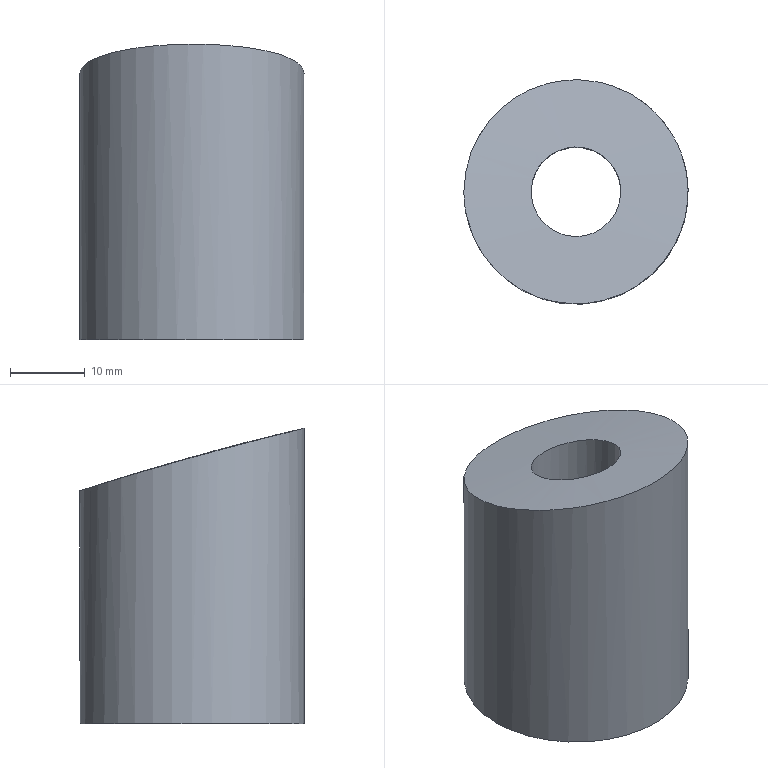Part | NX | features solid 2 | 1 solid | 4 faces | box 30.001 x 30 x 39.543 mm | volume 21121 mm3 | cylinder 2 | spline 1 | plane 1 | commonest cylinder face diameters 12 x1 30 x1
STEP:
#1=CARTESIAN_POINT('',(-749.977,149.178,105.858));
#2=VERTEX_POINT('',#1);
#3=CARTESIAN_POINT('',(-747.09,139.627,108.386));
#4=CARTESIAN_POINT('',(-751.538,149.125,105.94));
#5=CARTESIAN_POINT('',(-748.183,158.887,103.085));
#6=CARTESIAN_POINT('',(-741.846,163.791,101.556));
#7=CARTESIAN_POINT('',(-735.95,165.378,101.05));
#8=CARTESIAN_POINT('',(-729.883,164.528,101.326));
#9=CARTESIAN_POINT('',(-722.94,160.384,102.647));
#10=CARTESIAN_POINT('',(-718.485,151.039,105.473));
#11=CARTESIAN_POINT('',(-721.752,141.177,108.077));
#12=CARTESIAN_POINT('',(-728.129,136.217,109.277));
#13=CARTESIAN_POINT('',(-734.033,134.622,109.636));
#14=CARTESIAN_POINT('',(-740.114,135.47,109.413));
#15=CARTESIAN_POINT('',(-747.09,139.627,108.386));
#16=CARTESIAN_POINT('',(-751.538,149.125,105.94));
#17=CARTESIAN_POINT('',(-748.183,158.887,103.085));
#18=B_SPLINE_CURVE_WITH_KNOTS('',3,(#3,#4,#5,#6,#7,#8,#9,#10,#11,#12,#13,#14,#15,#16,#17),.UNSPECIFIED.,.T.,.F.,(1,1,1,1,1,1,1,1,1,1,1,1,1,1,1,1,1,1,1),(-0.02388,-0.01791,-0.01194,0.,0.01194,0.01791,0.02388,0.02986,0.03583,0.04777,0.05971,0.06568,0.07165,0.07762,0.0836,0.09554,0.1075,0.1135,0.1194),.UNSPECIFIED.);
#19=EDGE_CURVE('',#2,#2,#18,.T.);
#20=ORIENTED_EDGE('',*,*,#19,.T.);
#21=EDGE_LOOP('',(#20));
#22=FACE_BOUND('',#21,.T.);
#23=CARTESIAN_POINT('',(-750.,150.,70.));
#24=VERTEX_POINT('',#23);
#25=CARTESIAN_POINT('',(-735.,150.,70.));
#26=DIRECTION('',(0.,0.,-1.));
#27=DIRECTION('',(-1.,0.,0.));
#28=AXIS2_PLACEMENT_3D('',#25,#26,#27);
#29=CIRCLE('',#28,15.);
#30=EDGE_CURVE('',#24,#24,#29,.T.);
#31=ORIENTED_EDGE('',*,*,#30,.F.);
#32=EDGE_LOOP('',(#31));
#33=FACE_BOUND('',#32,.T.);
#34=CARTESIAN_POINT('',(-735.,150.,120.));
#35=DIRECTION('',(0.,0.,-1.));
#36=DIRECTION('',(-1.,0.,0.));
#37=AXIS2_PLACEMENT_3D('',#34,#35,#36);
#38=CYLINDRICAL_SURFACE('',#37,15.);
#39=ADVANCED_FACE('',(#22,#33),#38,.T.);
#40=CARTESIAN_POINT('',(-729.,150.,105.676));
#41=VERTEX_POINT('',#40);
#42=CARTESIAN_POINT('',(-730.23,154.633,104.356));
#43=CARTESIAN_POINT('',(-728.384,150.001,105.688));
#44=CARTESIAN_POINT('',(-730.235,145.362,106.945));
#45=CARTESIAN_POINT('',(-735.002,143.317,107.465));
#46=CARTESIAN_POINT('',(-739.777,145.37,106.918));
#47=CARTESIAN_POINT('',(-741.615,150.02,105.656));
#48=CARTESIAN_POINT('',(-739.764,154.633,104.342));
#49=CARTESIAN_POINT('',(-735.004,156.684,103.739));
#50=CARTESIAN_POINT('',(-730.23,154.633,104.356));
#51=CARTESIAN_POINT('',(-728.384,150.001,105.688));
#52=CARTESIAN_POINT('',(-730.235,145.362,106.945));
#53=B_SPLINE_CURVE_WITH_KNOTS('',3,(#42,#43,#44,#45,#46,#47,#48,#49,#50,#51,#52),.UNSPECIFIED.,.T.,.F.,(1,1,1,1,1,1,1,1,1,1,1,1,1,1,1),(-0.01433,-0.009554,-0.004777,0.,0.004777,0.009554,0.01433,0.01911,0.02389,0.02866,0.03344,0.03822,0.04299,0.04777,0.05255),.UNSPECIFIED.);
#54=EDGE_CURVE('',#41,#41,#53,.T.);
#55=ORIENTED_EDGE('',*,*,#54,.T.);
#56=EDGE_LOOP('',(#55));
#57=FACE_BOUND('',#56,.T.);
#58=ORIENTED_EDGE('',*,*,#19,.F.);
#59=EDGE_LOOP('',(#58));
#60=FACE_BOUND('',#59,.T.);
#61=CARTESIAN_POINT('',(-751.476,165.919,100.866));
#62=CARTESIAN_POINT('',(-750.684,155.902,104.088));
#63=CARTESIAN_POINT('',(-749.909,145.712,106.935));
#64=CARTESIAN_POINT('',(-749.151,135.347,109.408));
#65=CARTESIAN_POINT('',(-741.263,165.51,101.003));
#66=CARTESIAN_POINT('',(-740.466,155.482,104.226));
#67=CARTESIAN_POINT('',(-739.686,145.281,107.076));
#68=CARTESIAN_POINT('',(-738.924,134.905,109.55));
#69=CARTESIAN_POINT('',(-731.05,165.1,101.14));
#70=CARTESIAN_POINT('',(-730.248,155.062,104.365));
#71=CARTESIAN_POINT('',(-729.464,144.85,107.216));
#72=CARTESIAN_POINT('',(-728.698,134.463,109.692));
#73=CARTESIAN_POINT('',(-720.837,164.691,101.277));
#74=CARTESIAN_POINT('',(-720.031,154.642,104.504));
#75=CARTESIAN_POINT('',(-719.242,144.419,107.356));
#76=CARTESIAN_POINT('',(-718.471,134.021,109.834));
#77=B_SPLINE_SURFACE_WITH_KNOTS('',3,3,((#61,#62,#63,#64),(#65,#66,#67,#68),(#69,#70,#71,#72),(#73,#74,#75,#76)),.UNSPECIFIED.,.F.,.F.,.F.,(4,4),(4,4),(0.2165,0.6205),(0.479,0.7331),.UNSPECIFIED.);
#78=ADVANCED_FACE('',(#57,#60),#77,.F.);
#79=CARTESIAN_POINT('',(-729.,150.,70.));
#80=VERTEX_POINT('',#79);
#81=CARTESIAN_POINT('',(-735.,150.,70.));
#82=DIRECTION('',(0.,0.,1.));
#83=DIRECTION('',(1.,0.,0.));
#84=AXIS2_PLACEMENT_3D('',#81,#82,#83);
#85=CIRCLE('',#84,6.);
#86=EDGE_CURVE('',#80,#80,#85,.T.);
#87=ORIENTED_EDGE('',*,*,#86,.T.);
#88=EDGE_LOOP('',(#87));
#89=FACE_BOUND('',#88,.T.);
#90=ORIENTED_EDGE('',*,*,#30,.T.);
#91=EDGE_LOOP('',(#90));
#92=FACE_BOUND('',#91,.T.);
#93=CARTESIAN_POINT('',(-735.,150.,70.));
#94=DIRECTION('',(0.,0.,-1.));
#95=DIRECTION('',(-1.,0.,0.));
#96=AXIS2_PLACEMENT_3D('',#93,#94,#95);
#97=PLANE('',#96);
#98=ADVANCED_FACE('',(#89,#92),#97,.T.);
#99=ORIENTED_EDGE('',*,*,#86,.F.);
#100=EDGE_LOOP('',(#99));
#101=FACE_BOUND('',#100,.T.);
#102=ORIENTED_EDGE('',*,*,#54,.F.);
#103=EDGE_LOOP('',(#102));
#104=FACE_BOUND('',#103,.T.);
#105=CARTESIAN_POINT('',(-735.,150.,70.));
#106=DIRECTION('',(0.,0.,1.));
#107=DIRECTION('',(1.,0.,0.));
#108=AXIS2_PLACEMENT_3D('',#105,#106,#107);
#109=CYLINDRICAL_SURFACE('',#108,6.);
#110=ADVANCED_FACE('',(#101,#104),#109,.F.);
#111=CLOSED_SHELL('',(#39,#78,#98,#110));
#112=MANIFOLD_SOLID_BREP('',#111);
#113=(LENGTH_UNIT()NAMED_UNIT(*)SI_UNIT(.MILLI.,.METRE.));
#114=UNCERTAINTY_MEASURE_WITH_UNIT(LENGTH_MEASURE(0.0508),#113,'','');
#115=(NAMED_UNIT(*)PLANE_ANGLE_UNIT()SI_UNIT($,.RADIAN.));
#116=(NAMED_UNIT(*)SI_UNIT($,.STERADIAN.)SOLID_ANGLE_UNIT());
#117=(GEOMETRIC_REPRESENTATION_CONTEXT(3)GLOBAL_UNCERTAINTY_ASSIGNED_CONTEXT((#114))GLOBAL_UNIT_ASSIGNED_CONTEXT((#113,#115,#116))REPRESENTATION_CONTEXT('',''));
#118=ADVANCED_BREP_SHAPE_REPRESENTATION('',(#112),#117);